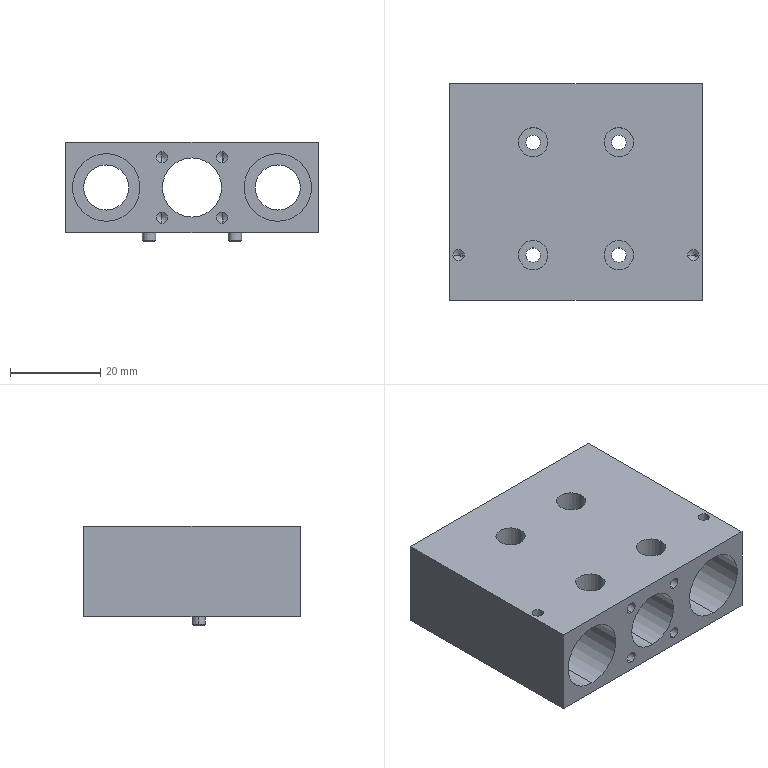NC program | NX | posted with a generic post | part box 56 x 48 x 22 mm
Whole program:
N10 G17 G21 G94 G90
(HOLE_MILLING , TOOL : D4)
N12 T04 M6
N14 G54
N16 G17 G0 G90 X-9.5 Y11. B0. C0. S9500 M3
N18 G43 Z30. H4
N20 Z0.5
N22 G94 G3 X-8.875 Y10.375 R0.625 F1400.
N24 X-8.25 Y11. R0.625
N26 X-8.25 Y11. Z0.1 I-1.25 J0.
N28 X-8.25 Y11. Z-0.3 I-1.25 J0.
N30 X-8.25 Y11. Z-0.7 I-1.25 J0.
N32 X-8.25 Y11. Z-1.1 I-1.25 J0.
N34 X-8.25 Y11. Z-1.5 I-1.25 J0.
N36 X-8.25 Y11. Z-1.9 I-1.25 J0.
N38 X-8.25 Y11. Z-2.3 I-1.25 J0.
N40 X-8.25 Y11. Z-2.7 I-1.25 J0.
N42 X-8.25 Y11. Z-3.1 I-1.25 J0.
N44 X-8.25 Y11. Z-3.5 I-1.25 J0.
N46 X-8.25 Y11. Z-3.9 I-1.25 J0.
N48 X-8.25 Y11. Z-4.3 I-1.25 J0.
N50 X-8.25 Y11. Z-4.7 I-1.25 J0.
N52 X-9.5 Y9.75 Z-5. R-1.25
N54 X-8.25 Y11. R1.25
N56 X-9.5 Y9.75 R-1.25
N58 X-8.875 Y10.375 R0.625
N60 X-9.5 Y11. R0.625
N62 G0 Z30.
N64 X9.5
N66 Z0.5
N68 G3 X10.125 Y10.375 R0.625
N70 X10.75 Y11. R0.625
N72 X10.75 Y11. Z0.1 I-1.25 J0.
N74 X10.75 Y11. Z-0.3 I-1.25 J0.
N76 X10.75 Y11. Z-0.7 I-1.25 J0.
N78 X10.75 Y11. Z-1.1 I-1.25 J0.
N80 X10.75 Y11. Z-1.5 I-1.25 J0.
N82 X10.75 Y11. Z-1.9 I-1.25 J0.
N84 X10.75 Y11. Z-2.3 I-1.25 J0.
N86 X10.75 Y11. Z-2.7 I-1.25 J0.
N88 X10.75 Y11. Z-3.1 I-1.25 J0.
N90 X10.75 Y11. Z-3.5 I-1.25 J0.
N92 X10.75 Y11. Z-3.9 I-1.25 J0.
N94 X10.75 Y11. Z-4.3 I-1.25 J0.
N96 X10.75 Y11. Z-4.7 I-1.25 J0.
N98 X9.5 Y9.75 Z-5. R-1.25
N100 X10.75 Y11. R1.25
N102 X9.5 Y9.75 R-1.25
N104 X10.125 Y10.375 R0.625
N106 X9.5 Y11. R0.625
N108 G0 Z30.
N110 X-9.5 Y-14.
N112 Z0.5
N114 G3 X-8.875 Y-14.625 R0.625
N116 X-8.25 Y-14. R0.625
N118 X-8.25 Y-14. Z0.1 I-1.25 J0.
N120 X-8.25 Y-14. Z-0.3 I-1.25 J0.
N122 X-8.25 Y-14. Z-0.7 I-1.25 J0.
N124 X-8.25 Y-14. Z-1.1 I-1.25 J0.
N126 X-8.25 Y-14. Z-1.5 I-1.25 J0.
N128 X-8.25 Y-14. Z-1.9 I-1.25 J0.
N130 X-8.25 Y-14. Z-2.3 I-1.25 J0.
N132 X-8.25 Y-14. Z-2.7 I-1.25 J0.
N134 X-8.25 Y-14. Z-3.1 I-1.25 J0.
N136 X-8.25 Y-14. Z-3.5 I-1.25 J0.
N138 X-8.25 Y-14. Z-3.9 I-1.25 J0.
N140 X-8.25 Y-14. Z-4.3 I-1.25 J0.
N142 X-8.25 Y-14. Z-4.7 I-1.25 J0.
N144 X-9.5 Y-15.25 Z-5. R-1.25
N146 X-8.25 Y-14. R1.25
N148 X-9.5 Y-15.25 R-1.25
N150 X-8.875 Y-14.625 R0.625
N152 X-9.5 Y-14. R0.625
N154 G0 Z30.
N156 X9.5
N158 Z0.5
N160 G3 X10.125 Y-14.625 R0.625
N162 X10.75 Y-14. R0.625
N164 X10.75 Y-14. Z0.1 I-1.25 J0.
N166 X10.75 Y-14. Z-0.3 I-1.25 J0.
N168 X10.75 Y-14. Z-0.7 I-1.25 J0.
N170 X10.75 Y-14. Z-1.1 I-1.25 J0.
N172 X10.75 Y-14. Z-1.5 I-1.25 J0.
N174 X10.75 Y-14. Z-1.9 I-1.25 J0.
N176 X10.75 Y-14. Z-2.3 I-1.25 J0.
N178 X10.75 Y-14. Z-2.7 I-1.25 J0.
N180 X10.75 Y-14. Z-3.1 I-1.25 J0.
N182 X10.75 Y-14. Z-3.5 I-1.25 J0.
N184 X10.75 Y-14. Z-3.9 I-1.25 J0.
N186 X10.75 Y-14. Z-4.3 I-1.25 J0.
N188 X10.75 Y-14. Z-4.7 I-1.25 J0.
N190 X9.5 Y-15.25 Z-5. R-1.25
N192 X10.75 Y-14. R1.25
N194 X9.5 Y-15.25 R-1.25
N196 X10.125 Y-14.625 R0.625
N198 X9.5 Y-14. R0.625
N200 G0 Z30.
N202 M5
N204 M2